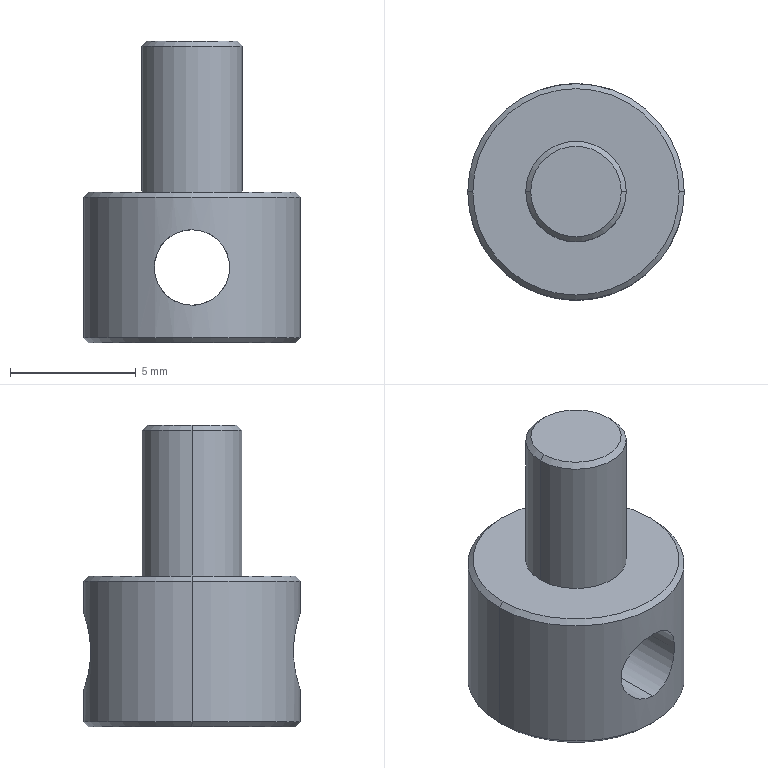Part | SolidWorks | features Chamfer 1, Extrusion 1, HoleWzd 1, ICE 1 | 1 solid | 15 faces | box 8.6 x 8.6 x 12 mm | volume 362.769 mm3 | cylinder 6 | cone 6 | plane 3 | commonest cylinder face diameters 3 x2 4 x2 8.6 x2
STEP:
#1=CARTESIAN_POINT('',(0.,-4.3,1.5));
#2=VERTEX_POINT('',#1);
#3=CARTESIAN_POINT('',(0.,-4.3,4.5));
#4=VERTEX_POINT('',#3);
#5=CARTESIAN_POINT('',(0.,-4.3,1.5));
#6=CARTESIAN_POINT('',(-0.1969,-4.3,1.5));
#7=CARTESIAN_POINT('',(-0.3956,-4.286,1.54));
#8=CARTESIAN_POINT('',(-0.6672,-4.249,1.653));
#9=CARTESIAN_POINT('',(-0.7549,-4.234,1.7));
#10=CARTESIAN_POINT('',(-0.9167,-4.202,1.809));
#11=CARTESIAN_POINT('',(-0.9918,-4.185,1.87));
#12=CARTESIAN_POINT('',(-1.2,-4.132,2.078));
#13=CARTESIAN_POINT('',(-1.309,-4.097,2.242));
#14=CARTESIAN_POINT('',(-1.423,-4.058,2.515));
#15=CARTESIAN_POINT('',(-1.451,-4.048,2.609));
#16=CARTESIAN_POINT('',(-1.49,-4.034,2.801));
#17=CARTESIAN_POINT('',(-1.5,-4.03,2.901));
#18=CARTESIAN_POINT('',(-1.5,-4.03,3.198));
#19=CARTESIAN_POINT('',(-1.46,-4.045,3.396));
#20=CARTESIAN_POINT('',(-1.309,-4.097,3.757));
#21=CARTESIAN_POINT('',(-1.198,-4.132,3.923));
#22=CARTESIAN_POINT('',(-0.9919,-4.185,4.129));
#23=CARTESIAN_POINT('',(-0.9154,-4.202,4.192));
#24=CARTESIAN_POINT('',(-0.7535,-4.234,4.301));
#25=CARTESIAN_POINT('',(-0.6677,-4.249,4.347));
#26=CARTESIAN_POINT('',(-0.4861,-4.273,4.422));
#27=CARTESIAN_POINT('',(-0.3906,-4.283,4.452));
#28=CARTESIAN_POINT('',(-0.198,-4.297,4.49));
#29=CARTESIAN_POINT('',(-0.09993,-4.3,4.5));
#30=CARTESIAN_POINT('',(0.,-4.3,4.5));
#31=B_SPLINE_CURVE_WITH_KNOTS('',3,(#5,#6,#7,#8,#9,#10,#11,#12,#13,#14,#15,#16,#17,#18,#19,#20,#21,#22,#23,#24,#25,#26,#27,#28,#29,#30),.UNSPECIFIED.,.F.,.F.,(4,2,2,2,2,2,2,2,2,2,2,2,4),(0.004727,0.005318,0.005613,0.005909,0.006499,0.006795,0.00709,0.007681,0.008272,0.008567,0.008862,0.009158,0.009453),.UNSPECIFIED.);
#32=EDGE_CURVE('',#2,#4,#31,.T.);
#33=ORIENTED_EDGE('',*,*,#32,.F.);
#34=CARTESIAN_POINT('',(0.,4.3,1.5));
#35=VERTEX_POINT('',#34);
#36=CARTESIAN_POINT('',(0.,5.,1.5));
#37=DIRECTION('',(0.,1.,0.));
#38=VECTOR('',#37,1000.);
#39=LINE('',#36,#38);
#40=EDGE_CURVE('',#2,#35,#39,.T.);
#41=ORIENTED_EDGE('',*,*,#40,.T.);
#42=CARTESIAN_POINT('',(0.,4.3,4.5));
#43=VERTEX_POINT('',#42);
#44=CARTESIAN_POINT('',(0.,4.3,4.5));
#45=CARTESIAN_POINT('',(-0.09996,4.3,4.5));
#46=CARTESIAN_POINT('',(-0.1981,4.297,4.49));
#47=CARTESIAN_POINT('',(-0.3909,4.283,4.451));
#48=CARTESIAN_POINT('',(-0.4866,4.273,4.422));
#49=CARTESIAN_POINT('',(-0.7587,4.236,4.309));
#50=CARTESIAN_POINT('',(-0.924,4.202,4.197));
#51=CARTESIAN_POINT('',(-1.198,4.132,3.923));
#52=CARTESIAN_POINT('',(-1.31,4.096,3.757));
#53=CARTESIAN_POINT('',(-1.422,4.058,3.487));
#54=CARTESIAN_POINT('',(-1.451,4.048,3.391));
#55=CARTESIAN_POINT('',(-1.49,4.034,3.197));
#56=CARTESIAN_POINT('',(-1.5,4.03,3.1));
#57=CARTESIAN_POINT('',(-1.5,4.03,2.902));
#58=CARTESIAN_POINT('',(-1.49,4.034,2.802));
#59=CARTESIAN_POINT('',(-1.451,4.048,2.609));
#60=CARTESIAN_POINT('',(-1.423,4.058,2.515));
#61=CARTESIAN_POINT('',(-1.309,4.097,2.241));
#62=CARTESIAN_POINT('',(-1.198,4.132,2.077));
#63=CARTESIAN_POINT('',(-0.9913,4.185,1.87));
#64=CARTESIAN_POINT('',(-0.9163,4.202,1.808));
#65=CARTESIAN_POINT('',(-0.7543,4.234,1.7));
#66=CARTESIAN_POINT('',(-0.6665,4.249,1.653));
#67=CARTESIAN_POINT('',(-0.3957,4.286,1.54));
#68=CARTESIAN_POINT('',(-0.1969,4.3,1.5));
#69=CARTESIAN_POINT('',(0.,4.3,1.5));
#70=B_SPLINE_CURVE_WITH_KNOTS('',3,(#44,#45,#46,#47,#48,#49,#50,#51,#52,#53,#54,#55,#56,#57,#58,#59,#60,#61,#62,#63,#64,#65,#66,#67,#68,#69),.UNSPECIFIED.,.F.,.F.,(4,2,2,2,2,2,2,2,2,2,2,2,4),(0.,0.0002954,0.0005909,0.001182,0.001773,0.002068,0.002364,0.002659,0.002954,0.003545,0.003841,0.004136,0.004727),.UNSPECIFIED.);
#71=EDGE_CURVE('',#43,#35,#70,.T.);
#72=ORIENTED_EDGE('',*,*,#71,.F.);
#73=CARTESIAN_POINT('',(0.,5.,4.5));
#74=DIRECTION('',(0.,1.,0.));
#75=VECTOR('',#74,1000.);
#76=LINE('',#73,#75);
#77=EDGE_CURVE('',#4,#43,#76,.T.);
#78=ORIENTED_EDGE('',*,*,#77,.F.);
#79=EDGE_LOOP('',(#33,#41,#72,#78));
#80=FACE_OUTER_BOUND('',#79,.T.);
#81=CARTESIAN_POINT('',(0.,5.,3.));
#82=DIRECTION('',(0.,1.,0.));
#83=DIRECTION('',(0.,0.,1.));
#84=AXIS2_PLACEMENT_3D('',#81,#82,#83);
#85=CYLINDRICAL_SURFACE('',#84,1.5);
#86=ADVANCED_FACE('',(#80),#85,.F.);
#87=CARTESIAN_POINT('',(1.8,0.,12.));
#88=VERTEX_POINT('',#87);
#89=CARTESIAN_POINT('',(-1.8,0.,12.));
#90=VERTEX_POINT('',#89);
#91=CARTESIAN_POINT('',(0.,0.,12.));
#92=DIRECTION('',(0.,0.,1.));
#93=DIRECTION('',(1.,0.,0.));
#94=AXIS2_PLACEMENT_3D('',#91,#92,#93);
#95=CIRCLE('',#94,1.8);
#96=EDGE_CURVE('',#88,#90,#95,.T.);
#97=ORIENTED_EDGE('',*,*,#96,.F.);
#98=CARTESIAN_POINT('',(2.,0.,11.8));
#99=VERTEX_POINT('',#98);
#100=CARTESIAN_POINT('',(1.8,0.,12.));
#101=DIRECTION('',(0.7071,0.,-0.7071));
#102=VECTOR('',#101,1000.);
#103=LINE('',#100,#102);
#104=EDGE_CURVE('',#88,#99,#103,.T.);
#105=ORIENTED_EDGE('',*,*,#104,.T.);
#106=CARTESIAN_POINT('',(-2.,0.,11.8));
#107=VERTEX_POINT('',#106);
#108=CARTESIAN_POINT('',(0.,0.,11.8));
#109=DIRECTION('',(0.,0.,-1.));
#110=DIRECTION('',(1.,0.,0.));
#111=AXIS2_PLACEMENT_3D('',#108,#109,#110);
#112=CIRCLE('',#111,2.);
#113=EDGE_CURVE('',#107,#99,#112,.T.);
#114=ORIENTED_EDGE('',*,*,#113,.F.);
#115=CARTESIAN_POINT('',(-1.8,0.,12.));
#116=DIRECTION('',(-0.7071,0.,-0.7071));
#117=VECTOR('',#116,1000.);
#118=LINE('',#115,#117);
#119=EDGE_CURVE('',#90,#107,#118,.T.);
#120=ORIENTED_EDGE('',*,*,#119,.F.);
#121=EDGE_LOOP('',(#97,#105,#114,#120));
#122=FACE_OUTER_BOUND('',#121,.T.);
#123=CARTESIAN_POINT('',(0.,0.,12.));
#124=DIRECTION('',(0.,0.,-1.));
#125=DIRECTION('',(-1.,0.,0.));
#126=AXIS2_PLACEMENT_3D('',#123,#124,#125);
#127=CONICAL_SURFACE('',#126,1.8,0.7854);
#128=ADVANCED_FACE('',(#122),#127,.T.);
#129=CARTESIAN_POINT('',(4.1,0.,6.));
#130=VERTEX_POINT('',#129);
#131=CARTESIAN_POINT('',(-4.1,0.,6.));
#132=VERTEX_POINT('',#131);
#133=CARTESIAN_POINT('',(0.,0.,6.));
#134=DIRECTION('',(0.,0.,1.));
#135=DIRECTION('',(1.,0.,0.));
#136=AXIS2_PLACEMENT_3D('',#133,#134,#135);
#137=CIRCLE('',#136,4.1);
#138=EDGE_CURVE('',#130,#132,#137,.T.);
#139=ORIENTED_EDGE('',*,*,#138,.F.);
#140=CARTESIAN_POINT('',(4.3,0.,5.8));
#141=VERTEX_POINT('',#140);
#142=CARTESIAN_POINT('',(4.1,0.,6.));
#143=DIRECTION('',(0.7071,0.,-0.7071));
#144=VECTOR('',#143,1000.);
#145=LINE('',#142,#144);
#146=EDGE_CURVE('',#130,#141,#145,.T.);
#147=ORIENTED_EDGE('',*,*,#146,.T.);
#148=CARTESIAN_POINT('',(-4.3,0.,5.8));
#149=VERTEX_POINT('',#148);
#150=CARTESIAN_POINT('',(0.,0.,5.8));
#151=DIRECTION('',(0.,0.,-1.));
#152=DIRECTION('',(1.,0.,0.));
#153=AXIS2_PLACEMENT_3D('',#150,#151,#152);
#154=CIRCLE('',#153,4.3);
#155=EDGE_CURVE('',#149,#141,#154,.T.);
#156=ORIENTED_EDGE('',*,*,#155,.F.);
#157=CARTESIAN_POINT('',(-4.1,0.,6.));
#158=DIRECTION('',(-0.7071,0.,-0.7071));
#159=VECTOR('',#158,1000.);
#160=LINE('',#157,#159);
#161=EDGE_CURVE('',#132,#149,#160,.T.);
#162=ORIENTED_EDGE('',*,*,#161,.F.);
#163=EDGE_LOOP('',(#139,#147,#156,#162));
#164=FACE_OUTER_BOUND('',#163,.T.);
#165=CARTESIAN_POINT('',(0.,0.,6.));
#166=DIRECTION('',(0.,0.,-1.));
#167=DIRECTION('',(-1.,0.,0.));
#168=AXIS2_PLACEMENT_3D('',#165,#166,#167);
#169=CONICAL_SURFACE('',#168,4.1,0.7854);
#170=ADVANCED_FACE('',(#164),#169,.T.);
#171=CARTESIAN_POINT('',(-4.1,0.,0.));
#172=VERTEX_POINT('',#171);
#173=CARTESIAN_POINT('',(4.1,0.,0.));
#174=VERTEX_POINT('',#173);
#175=CARTESIAN_POINT('',(0.,0.,0.));
#176=DIRECTION('',(0.,0.,-1.));
#177=DIRECTION('',(1.,0.,0.));
#178=AXIS2_PLACEMENT_3D('',#175,#176,#177);
#179=CIRCLE('',#178,4.1);
#180=EDGE_CURVE('',#172,#174,#179,.T.);
#181=ORIENTED_EDGE('',*,*,#180,.F.);
#182=CARTESIAN_POINT('',(-4.3,0.,0.2));
#183=VERTEX_POINT('',#182);
#184=CARTESIAN_POINT('',(-4.3,0.,0.2));
#185=DIRECTION('',(-0.7071,0.,0.7071));
#186=VECTOR('',#185,1000.);
#187=LINE('',#184,#186);
#188=EDGE_CURVE('',#172,#183,#187,.T.);
#189=ORIENTED_EDGE('',*,*,#188,.T.);
#190=CARTESIAN_POINT('',(4.3,0.,0.2));
#191=VERTEX_POINT('',#190);
#192=CARTESIAN_POINT('',(0.,0.,0.2));
#193=DIRECTION('',(0.,0.,1.));
#194=DIRECTION('',(1.,0.,0.));
#195=AXIS2_PLACEMENT_3D('',#192,#193,#194);
#196=CIRCLE('',#195,4.3);
#197=EDGE_CURVE('',#191,#183,#196,.T.);
#198=ORIENTED_EDGE('',*,*,#197,.F.);
#199=CARTESIAN_POINT('',(4.3,0.,0.2));
#200=DIRECTION('',(0.7071,0.,0.7071));
#201=VECTOR('',#200,1000.);
#202=LINE('',#199,#201);
#203=EDGE_CURVE('',#174,#191,#202,.T.);
#204=ORIENTED_EDGE('',*,*,#203,.F.);
#205=EDGE_LOOP('',(#181,#189,#198,#204));
#206=FACE_OUTER_BOUND('',#205,.T.);
#207=CARTESIAN_POINT('',(0.,0.,0.2));
#208=DIRECTION('',(0.,0.,1.));
#209=DIRECTION('',(1.,0.,0.));
#210=AXIS2_PLACEMENT_3D('',#207,#208,#209);
#211=CONICAL_SURFACE('',#210,4.3,0.7854);
#212=ADVANCED_FACE('',(#206),#211,.T.);
#213=ORIENTED_EDGE('',*,*,#113,.T.);
#214=CARTESIAN_POINT('',(2.,0.,6.));
#215=VERTEX_POINT('',#214);
#216=CARTESIAN_POINT('',(2.,0.,12.));
#217=DIRECTION('',(0.,0.,-1.));
#218=VECTOR('',#217,1000.);
#219=LINE('',#216,#218);
#220=EDGE_CURVE('',#99,#215,#219,.T.);
#221=ORIENTED_EDGE('',*,*,#220,.T.);
#222=CARTESIAN_POINT('',(-2.,0.,6.));
#223=VERTEX_POINT('',#222);
#224=CARTESIAN_POINT('',(0.,0.,6.));
#225=DIRECTION('',(0.,0.,1.));
#226=DIRECTION('',(1.,0.,0.));
#227=AXIS2_PLACEMENT_3D('',#224,#225,#226);
#228=CIRCLE('',#227,2.);
#229=EDGE_CURVE('',#215,#223,#228,.T.);
#230=ORIENTED_EDGE('',*,*,#229,.T.);
#231=CARTESIAN_POINT('',(-2.,0.,12.));
#232=DIRECTION('',(0.,0.,-1.));
#233=VECTOR('',#232,1000.);
#234=LINE('',#231,#233);
#235=EDGE_CURVE('',#107,#223,#234,.T.);
#236=ORIENTED_EDGE('',*,*,#235,.F.);
#237=EDGE_LOOP('',(#213,#221,#230,#236));
#238=FACE_OUTER_BOUND('',#237,.T.);
#239=CARTESIAN_POINT('',(0.,0.,12.));
#240=DIRECTION('',(0.,0.,-1.));
#241=DIRECTION('',(-1.,0.,0.));
#242=AXIS2_PLACEMENT_3D('',#239,#240,#241);
#243=CYLINDRICAL_SURFACE('',#242,2.);
#244=ADVANCED_FACE('',(#238),#243,.T.);
#245=ORIENTED_EDGE('',*,*,#71,.T.);
#246=CARTESIAN_POINT('',(0.,4.3,1.5));
#247=CARTESIAN_POINT('',(0.1969,4.3,1.5));
#248=CARTESIAN_POINT('',(0.3956,4.286,1.54));
#249=CARTESIAN_POINT('',(0.6672,4.249,1.653));
#250=CARTESIAN_POINT('',(0.7549,4.234,1.7));
#251=CARTESIAN_POINT('',(0.9167,4.202,1.809));
#252=CARTESIAN_POINT('',(0.9918,4.185,1.87));
#253=CARTESIAN_POINT('',(1.2,4.132,2.078));
#254=CARTESIAN_POINT('',(1.309,4.097,2.242));
#255=CARTESIAN_POINT('',(1.423,4.058,2.515));
#256=CARTESIAN_POINT('',(1.451,4.048,2.609));
#257=CARTESIAN_POINT('',(1.49,4.034,2.801));
#258=CARTESIAN_POINT('',(1.5,4.03,2.901));
#259=CARTESIAN_POINT('',(1.5,4.03,3.198));
#260=CARTESIAN_POINT('',(1.46,4.045,3.396));
#261=CARTESIAN_POINT('',(1.309,4.097,3.757));
#262=CARTESIAN_POINT('',(1.198,4.132,3.923));
#263=CARTESIAN_POINT('',(0.9919,4.185,4.129));
#264=CARTESIAN_POINT('',(0.9154,4.202,4.192));
#265=CARTESIAN_POINT('',(0.7535,4.234,4.301));
#266=CARTESIAN_POINT('',(0.6677,4.249,4.347));
#267=CARTESIAN_POINT('',(0.4861,4.273,4.422));
#268=CARTESIAN_POINT('',(0.3906,4.283,4.452));
#269=CARTESIAN_POINT('',(0.198,4.297,4.49));
#270=CARTESIAN_POINT('',(0.09993,4.3,4.5));
#271=CARTESIAN_POINT('',(0.,4.3,4.5));
#272=B_SPLINE_CURVE_WITH_KNOTS('',3,(#246,#247,#248,#249,#250,#251,#252,#253,#254,#255,#256,#257,#258,#259,#260,#261,#262,#263,#264,#265,#266,#267,#268,#269,#270,#271),.UNSPECIFIED.,.F.,.F.,(4,2,2,2,2,2,2,2,2,2,2,2,4),(0.004727,0.005318,0.005613,0.005909,0.006499,0.006795,0.00709,0.007681,0.008272,0.008567,0.008862,0.009158,0.009453),.UNSPECIFIED.);
#273=EDGE_CURVE('',#35,#43,#272,.T.);
#274=ORIENTED_EDGE('',*,*,#273,.T.);
#275=EDGE_LOOP('',(#245,#274));
#276=FACE_BOUND('',#275,.T.);
#277=ORIENTED_EDGE('',*,*,#155,.T.);
#278=CARTESIAN_POINT('',(4.3,0.,6.));
#279=DIRECTION('',(0.,0.,-1.));
#280=VECTOR('',#279,1000.);
#281=LINE('',#278,#280);
#282=EDGE_CURVE('',#141,#191,#281,.T.);
#283=ORIENTED_EDGE('',*,*,#282,.T.);
#284=ORIENTED_EDGE('',*,*,#197,.T.);
#285=CARTESIAN_POINT('',(-4.3,0.,6.));
#286=DIRECTION('',(0.,0.,-1.));
#287=VECTOR('',#286,1000.);
#288=LINE('',#285,#287);
#289=EDGE_CURVE('',#149,#183,#288,.T.);
#290=ORIENTED_EDGE('',*,*,#289,.F.);
#291=EDGE_LOOP('',(#277,#283,#284,#290));
#292=FACE_OUTER_BOUND('',#291,.T.);
#293=CARTESIAN_POINT('',(0.,0.,6.));
#294=DIRECTION('',(0.,0.,-1.));
#295=DIRECTION('',(-1.,0.,0.));
#296=AXIS2_PLACEMENT_3D('',#293,#294,#295);
#297=CYLINDRICAL_SURFACE('',#296,4.3);
#298=ADVANCED_FACE('',(#276,#292),#297,.T.);
#299=ORIENTED_EDGE('',*,*,#282,.F.);
#300=CARTESIAN_POINT('',(0.,0.,5.8));
#301=DIRECTION('',(0.,0.,-1.));
#302=DIRECTION('',(1.,0.,0.));
#303=AXIS2_PLACEMENT_3D('',#300,#301,#302);
#304=CIRCLE('',#303,4.3);
#305=EDGE_CURVE('',#141,#149,#304,.T.);
#306=ORIENTED_EDGE('',*,*,#305,.T.);
#307=ORIENTED_EDGE('',*,*,#289,.T.);
#308=CARTESIAN_POINT('',(0.,0.,0.2));
#309=DIRECTION('',(0.,0.,1.));
#310=DIRECTION('',(1.,0.,0.));
#311=AXIS2_PLACEMENT_3D('',#308,#309,#310);
#312=CIRCLE('',#311,4.3);
#313=EDGE_CURVE('',#183,#191,#312,.T.);
#314=ORIENTED_EDGE('',*,*,#313,.T.);
#315=EDGE_LOOP('',(#299,#306,#307,#314));
#316=FACE_OUTER_BOUND('',#315,.T.);
#317=CARTESIAN_POINT('',(0.,-4.3,4.5));
#318=CARTESIAN_POINT('',(0.09996,-4.3,4.5));
#319=CARTESIAN_POINT('',(0.1981,-4.297,4.49));
#320=CARTESIAN_POINT('',(0.3909,-4.283,4.451));
#321=CARTESIAN_POINT('',(0.4866,-4.273,4.422));
#322=CARTESIAN_POINT('',(0.7587,-4.236,4.309));
#323=CARTESIAN_POINT('',(0.924,-4.202,4.197));
#324=CARTESIAN_POINT('',(1.198,-4.132,3.923));
#325=CARTESIAN_POINT('',(1.31,-4.096,3.757));
#326=CARTESIAN_POINT('',(1.422,-4.058,3.487));
#327=CARTESIAN_POINT('',(1.451,-4.048,3.391));
#328=CARTESIAN_POINT('',(1.49,-4.034,3.197));
#329=CARTESIAN_POINT('',(1.5,-4.03,3.1));
#330=CARTESIAN_POINT('',(1.5,-4.03,2.902));
#331=CARTESIAN_POINT('',(1.49,-4.034,2.802));
#332=CARTESIAN_POINT('',(1.451,-4.048,2.609));
#333=CARTESIAN_POINT('',(1.423,-4.058,2.515));
#334=CARTESIAN_POINT('',(1.309,-4.097,2.241));
#335=CARTESIAN_POINT('',(1.198,-4.132,2.077));
#336=CARTESIAN_POINT('',(0.9913,-4.185,1.87));
#337=CARTESIAN_POINT('',(0.9163,-4.202,1.808));
#338=CARTESIAN_POINT('',(0.7543,-4.234,1.7));
#339=CARTESIAN_POINT('',(0.6665,-4.249,1.653));
#340=CARTESIAN_POINT('',(0.3957,-4.286,1.54));
#341=CARTESIAN_POINT('',(0.1969,-4.3,1.5));
#342=CARTESIAN_POINT('',(0.,-4.3,1.5));
#343=B_SPLINE_CURVE_WITH_KNOTS('',3,(#317,#318,#319,#320,#321,#322,#323,#324,#325,#326,#327,#328,#329,#330,#331,#332,#333,#334,#335,#336,#337,#338,#339,#340,#341,#342),.UNSPECIFIED.,.F.,.F.,(4,2,2,2,2,2,2,2,2,2,2,2,4),(0.,0.0002954,0.0005909,0.001182,0.001773,0.002068,0.002364,0.002659,0.002954,0.003545,0.003841,0.004136,0.004727),.UNSPECIFIED.);
#344=EDGE_CURVE('',#4,#2,#343,.T.);
#345=ORIENTED_EDGE('',*,*,#344,.T.);
#346=ORIENTED_EDGE('',*,*,#32,.T.);
#347=EDGE_LOOP('',(#345,#346));
#348=FACE_BOUND('',#347,.T.);
#349=CARTESIAN_POINT('',(0.,0.,6.));
#350=DIRECTION('',(0.,0.,-1.));
#351=DIRECTION('',(-1.,0.,0.));
#352=AXIS2_PLACEMENT_3D('',#349,#350,#351);
#353=CYLINDRICAL_SURFACE('',#352,4.3);
#354=ADVANCED_FACE('',(#316,#348),#353,.T.);
#355=CARTESIAN_POINT('',(0.,0.,6.));
#356=DIRECTION('',(0.,0.,1.));
#357=DIRECTION('',(1.,0.,0.));
#358=AXIS2_PLACEMENT_3D('',#355,#356,#357);
#359=CIRCLE('',#358,4.1);
#360=EDGE_CURVE('',#132,#130,#359,.T.);
#361=ORIENTED_EDGE('',*,*,#360,.T.);
#362=ORIENTED_EDGE('',*,*,#138,.T.);
#363=EDGE_LOOP('',(#361,#362));
#364=FACE_OUTER_BOUND('',#363,.T.);
#365=CARTESIAN_POINT('',(0.,0.,6.));
#366=DIRECTION('',(0.,0.,1.));
#367=DIRECTION('',(1.,0.,0.));
#368=AXIS2_PLACEMENT_3D('',#365,#366,#367);
#369=CIRCLE('',#368,2.);
#370=EDGE_CURVE('',#223,#215,#369,.T.);
#371=ORIENTED_EDGE('',*,*,#370,.F.);
#372=ORIENTED_EDGE('',*,*,#229,.F.);
#373=EDGE_LOOP('',(#371,#372));
#374=FACE_BOUND('',#373,.T.);
#375=CARTESIAN_POINT('',(0.,0.,6.));
#376=DIRECTION('',(0.,0.,1.));
#377=DIRECTION('',(1.,0.,0.));
#378=AXIS2_PLACEMENT_3D('',#375,#376,#377);
#379=PLANE('',#378);
#380=ADVANCED_FACE('',(#364,#374),#379,.T.);
#381=CARTESIAN_POINT('',(0.,0.,0.));
#382=DIRECTION('',(0.,0.,-1.));
#383=DIRECTION('',(1.,0.,0.));
#384=AXIS2_PLACEMENT_3D('',#381,#382,#383);
#385=CIRCLE('',#384,4.1);
#386=EDGE_CURVE('',#174,#172,#385,.T.);
#387=ORIENTED_EDGE('',*,*,#386,.T.);
#388=ORIENTED_EDGE('',*,*,#180,.T.);
#389=EDGE_LOOP('',(#387,#388));
#390=FACE_OUTER_BOUND('',#389,.T.);
#391=CARTESIAN_POINT('',(0.,0.,0.));
#392=DIRECTION('',(0.,0.,1.));
#393=DIRECTION('',(1.,0.,0.));
#394=AXIS2_PLACEMENT_3D('',#391,#392,#393);
#395=PLANE('',#394);
#396=ADVANCED_FACE('',(#390),#395,.F.);
#397=ORIENTED_EDGE('',*,*,#220,.F.);
#398=CARTESIAN_POINT('',(0.,0.,11.8));
#399=DIRECTION('',(0.,0.,-1.));
#400=DIRECTION('',(1.,0.,0.));
#401=AXIS2_PLACEMENT_3D('',#398,#399,#400);
#402=CIRCLE('',#401,2.);
#403=EDGE_CURVE('',#99,#107,#402,.T.);
#404=ORIENTED_EDGE('',*,*,#403,.T.);
#405=ORIENTED_EDGE('',*,*,#235,.T.);
#406=ORIENTED_EDGE('',*,*,#370,.T.);
#407=EDGE_LOOP('',(#397,#404,#405,#406));
#408=FACE_OUTER_BOUND('',#407,.T.);
#409=CARTESIAN_POINT('',(0.,0.,12.));
#410=DIRECTION('',(0.,0.,-1.));
#411=DIRECTION('',(-1.,0.,0.));
#412=AXIS2_PLACEMENT_3D('',#409,#410,#411);
#413=CYLINDRICAL_SURFACE('',#412,2.);
#414=ADVANCED_FACE('',(#408),#413,.T.);
#415=CARTESIAN_POINT('',(0.,0.,12.));
#416=DIRECTION('',(0.,0.,1.));
#417=DIRECTION('',(1.,0.,0.));
#418=AXIS2_PLACEMENT_3D('',#415,#416,#417);
#419=CIRCLE('',#418,1.8);
#420=EDGE_CURVE('',#90,#88,#419,.T.);
#421=ORIENTED_EDGE('',*,*,#420,.T.);
#422=ORIENTED_EDGE('',*,*,#96,.T.);
#423=EDGE_LOOP('',(#421,#422));
#424=FACE_OUTER_BOUND('',#423,.T.);
#425=CARTESIAN_POINT('',(0.,0.,12.));
#426=DIRECTION('',(0.,0.,1.));
#427=DIRECTION('',(1.,0.,0.));
#428=AXIS2_PLACEMENT_3D('',#425,#426,#427);
#429=PLANE('',#428);
#430=ADVANCED_FACE('',(#424),#429,.T.);
#431=ORIENTED_EDGE('',*,*,#188,.F.);
#432=ORIENTED_EDGE('',*,*,#386,.F.);
#433=ORIENTED_EDGE('',*,*,#203,.T.);
#434=ORIENTED_EDGE('',*,*,#313,.F.);
#435=EDGE_LOOP('',(#431,#432,#433,#434));
#436=FACE_OUTER_BOUND('',#435,.T.);
#437=CARTESIAN_POINT('',(0.,0.,0.2));
#438=DIRECTION('',(0.,0.,1.));
#439=DIRECTION('',(1.,0.,0.));
#440=AXIS2_PLACEMENT_3D('',#437,#438,#439);
#441=CONICAL_SURFACE('',#440,4.3,0.7854);
#442=ADVANCED_FACE('',(#436),#441,.T.);
#443=ORIENTED_EDGE('',*,*,#146,.F.);
#444=ORIENTED_EDGE('',*,*,#360,.F.);
#445=ORIENTED_EDGE('',*,*,#161,.T.);
#446=ORIENTED_EDGE('',*,*,#305,.F.);
#447=EDGE_LOOP('',(#443,#444,#445,#446));
#448=FACE_OUTER_BOUND('',#447,.T.);
#449=CARTESIAN_POINT('',(0.,0.,6.));
#450=DIRECTION('',(0.,0.,-1.));
#451=DIRECTION('',(-1.,0.,0.));
#452=AXIS2_PLACEMENT_3D('',#449,#450,#451);
#453=CONICAL_SURFACE('',#452,4.1,0.7854);
#454=ADVANCED_FACE('',(#448),#453,.T.);
#455=ORIENTED_EDGE('',*,*,#104,.F.);
#456=ORIENTED_EDGE('',*,*,#420,.F.);
#457=ORIENTED_EDGE('',*,*,#119,.T.);
#458=ORIENTED_EDGE('',*,*,#403,.F.);
#459=EDGE_LOOP('',(#455,#456,#457,#458));
#460=FACE_OUTER_BOUND('',#459,.T.);
#461=CARTESIAN_POINT('',(0.,0.,12.));
#462=DIRECTION('',(0.,0.,-1.));
#463=DIRECTION('',(-1.,0.,0.));
#464=AXIS2_PLACEMENT_3D('',#461,#462,#463);
#465=CONICAL_SURFACE('',#464,1.8,0.7854);
#466=ADVANCED_FACE('',(#460),#465,.T.);
#467=ORIENTED_EDGE('',*,*,#40,.F.);
#468=ORIENTED_EDGE('',*,*,#344,.F.);
#469=ORIENTED_EDGE('',*,*,#77,.T.);
#470=ORIENTED_EDGE('',*,*,#273,.F.);
#471=EDGE_LOOP('',(#467,#468,#469,#470));
#472=FACE_OUTER_BOUND('',#471,.T.);
#473=CARTESIAN_POINT('',(0.,5.,3.));
#474=DIRECTION('',(0.,1.,0.));
#475=DIRECTION('',(0.,0.,1.));
#476=AXIS2_PLACEMENT_3D('',#473,#474,#475);
#477=CYLINDRICAL_SURFACE('',#476,1.5);
#478=ADVANCED_FACE('',(#472),#477,.F.);
#479=CLOSED_SHELL('',(#86,#128,#170,#212,#244,#298,#354,#380,#396,#414,#430,#442,#454,#466,#478));
#480=MANIFOLD_SOLID_BREP('',#479);
#481=CARTESIAN_POINT('',(0.,0.,0.));
#482=DIRECTION('',(0.,0.,1.));
#483=DIRECTION('',(1.,0.,0.));
#484=AXIS2_PLACEMENT_3D('',#481,#482,#483);
#485=(LENGTH_UNIT()NAMED_UNIT(*)SI_UNIT(.MILLI.,.METRE.));
#486=UNCERTAINTY_MEASURE_WITH_UNIT(LENGTH_MEASURE(0.00001),#485,'','');
#487=(NAMED_UNIT(*)PLANE_ANGLE_UNIT()SI_UNIT($,.RADIAN.));
#488=(NAMED_UNIT(*)SI_UNIT($,.STERADIAN.)SOLID_ANGLE_UNIT());
#489=(GEOMETRIC_REPRESENTATION_CONTEXT(3)GLOBAL_UNCERTAINTY_ASSIGNED_CONTEXT((#486))GLOBAL_UNIT_ASSIGNED_CONTEXT((#485,#487,#488))REPRESENTATION_CONTEXT('',''));
#490=ADVANCED_BREP_SHAPE_REPRESENTATION('',(#480,#484),#489);